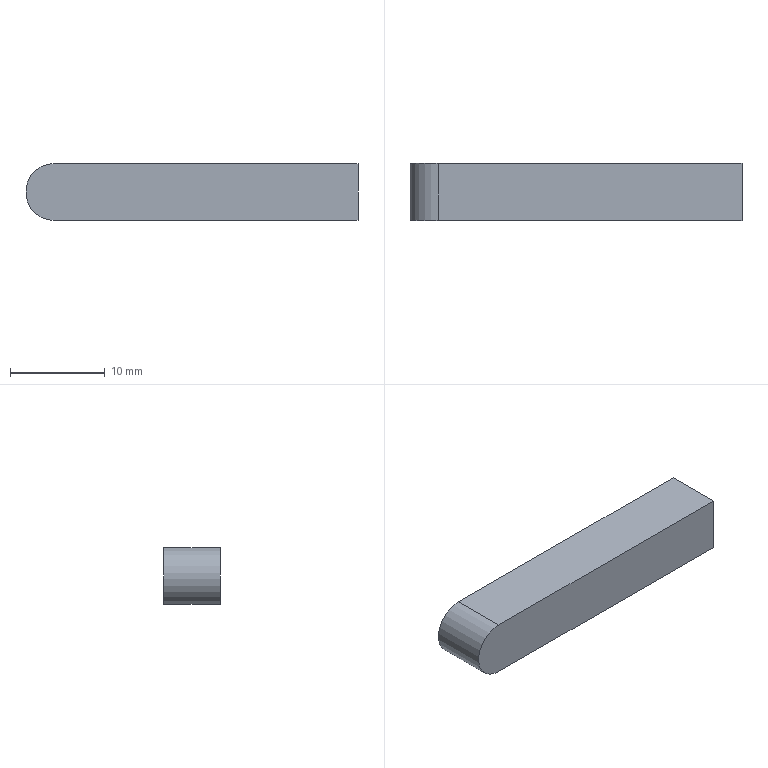Part | STEP file | G3L22N30-MM02TNNTNXH6-Part-5 | 1 solid | 6 faces | box 35 x 6 x 6 mm | volume 1237 mm3 | plane 5 | cylinder 1 | commonest cylinder face diameters 6 x1
STEP:
#1=CARTESIAN_POINT('',(40.,7.5,-3.));
#2=VERTEX_POINT('',#1);
#3=CARTESIAN_POINT('',(8.,7.5,-3.));
#4=VERTEX_POINT('',#3);
#5=CARTESIAN_POINT('',(40.,7.5,-3.));
#6=DIRECTION('',(-1.,0.,0.));
#7=VECTOR('',#6,1000.);
#8=LINE('',#5,#7);
#9=EDGE_CURVE('',#2,#4,#8,.T.);
#10=ORIENTED_EDGE('',*,*,#9,.T.);
#11=CARTESIAN_POINT('',(8.,13.5,-3.));
#12=VERTEX_POINT('',#11);
#13=CARTESIAN_POINT('',(8.,13.5,-3.));
#14=DIRECTION('',(0.,-1.,0.));
#15=VECTOR('',#14,1000.);
#16=LINE('',#13,#15);
#17=EDGE_CURVE('',#12,#4,#16,.T.);
#18=ORIENTED_EDGE('',*,*,#17,.F.);
#19=CARTESIAN_POINT('',(40.,13.5,-3.));
#20=VERTEX_POINT('',#19);
#21=CARTESIAN_POINT('',(40.,13.5,-3.));
#22=DIRECTION('',(-1.,0.,0.));
#23=VECTOR('',#22,1000.);
#24=LINE('',#21,#23);
#25=EDGE_CURVE('',#20,#12,#24,.T.);
#26=ORIENTED_EDGE('',*,*,#25,.F.);
#27=CARTESIAN_POINT('',(40.,13.5,-3.));
#28=DIRECTION('',(0.,-1.,0.));
#29=VECTOR('',#28,1000.);
#30=LINE('',#27,#29);
#31=EDGE_CURVE('',#20,#2,#30,.T.);
#32=ORIENTED_EDGE('',*,*,#31,.T.);
#33=EDGE_LOOP('',(#10,#18,#26,#32));
#34=FACE_OUTER_BOUND('',#33,.T.);
#35=CARTESIAN_POINT('',(40.,13.5,-3.));
#36=DIRECTION('',(0.,0.,1.));
#37=DIRECTION('',(1.,0.,0.));
#38=AXIS2_PLACEMENT_3D('',#35,#36,#37);
#39=PLANE('',#38);
#40=ADVANCED_FACE('',(#34),#39,.F.);
#41=CARTESIAN_POINT('',(8.,7.5,3.));
#42=VERTEX_POINT('',#41);
#43=CARTESIAN_POINT('',(8.,7.5,0.));
#44=DIRECTION('',(0.,1.,0.));
#45=DIRECTION('',(1.,0.,0.));
#46=AXIS2_PLACEMENT_3D('',#43,#44,#45);
#47=CIRCLE('',#46,3.);
#48=EDGE_CURVE('',#4,#42,#47,.T.);
#49=ORIENTED_EDGE('',*,*,#48,.T.);
#50=CARTESIAN_POINT('',(8.,13.5,3.));
#51=VERTEX_POINT('',#50);
#52=CARTESIAN_POINT('',(8.,13.5,3.));
#53=DIRECTION('',(0.,-1.,0.));
#54=VECTOR('',#53,1000.);
#55=LINE('',#52,#54);
#56=EDGE_CURVE('',#51,#42,#55,.T.);
#57=ORIENTED_EDGE('',*,*,#56,.F.);
#58=CARTESIAN_POINT('',(8.,13.5,0.));
#59=DIRECTION('',(0.,1.,0.));
#60=DIRECTION('',(1.,0.,0.));
#61=AXIS2_PLACEMENT_3D('',#58,#59,#60);
#62=CIRCLE('',#61,3.);
#63=EDGE_CURVE('',#12,#51,#62,.T.);
#64=ORIENTED_EDGE('',*,*,#63,.F.);
#65=ORIENTED_EDGE('',*,*,#17,.T.);
#66=EDGE_LOOP('',(#49,#57,#64,#65));
#67=FACE_OUTER_BOUND('',#66,.T.);
#68=CARTESIAN_POINT('',(8.,13.5,0.));
#69=DIRECTION('',(0.,-1.,0.));
#70=DIRECTION('',(0.,0.,-1.));
#71=AXIS2_PLACEMENT_3D('',#68,#69,#70);
#72=CYLINDRICAL_SURFACE('',#71,3.);
#73=ADVANCED_FACE('',(#67),#72,.T.);
#74=CARTESIAN_POINT('',(40.,7.5,3.));
#75=VERTEX_POINT('',#74);
#76=CARTESIAN_POINT('',(8.,7.5,3.));
#77=DIRECTION('',(1.,0.,0.));
#78=VECTOR('',#77,1000.);
#79=LINE('',#76,#78);
#80=EDGE_CURVE('',#42,#75,#79,.T.);
#81=ORIENTED_EDGE('',*,*,#80,.T.);
#82=CARTESIAN_POINT('',(40.,13.5,3.));
#83=VERTEX_POINT('',#82);
#84=CARTESIAN_POINT('',(40.,13.5,3.));
#85=DIRECTION('',(0.,-1.,0.));
#86=VECTOR('',#85,1000.);
#87=LINE('',#84,#86);
#88=EDGE_CURVE('',#83,#75,#87,.T.);
#89=ORIENTED_EDGE('',*,*,#88,.F.);
#90=CARTESIAN_POINT('',(8.,13.5,3.));
#91=DIRECTION('',(1.,0.,0.));
#92=VECTOR('',#91,1000.);
#93=LINE('',#90,#92);
#94=EDGE_CURVE('',#51,#83,#93,.T.);
#95=ORIENTED_EDGE('',*,*,#94,.F.);
#96=ORIENTED_EDGE('',*,*,#56,.T.);
#97=EDGE_LOOP('',(#81,#89,#95,#96));
#98=FACE_OUTER_BOUND('',#97,.T.);
#99=CARTESIAN_POINT('',(8.,13.5,3.));
#100=DIRECTION('',(0.,0.,-1.));
#101=DIRECTION('',(-1.,0.,0.));
#102=AXIS2_PLACEMENT_3D('',#99,#100,#101);
#103=PLANE('',#102);
#104=ADVANCED_FACE('',(#98),#103,.F.);
#105=CARTESIAN_POINT('',(40.,7.5,3.));
#106=DIRECTION('',(0.,0.,-1.));
#107=VECTOR('',#106,1000.);
#108=LINE('',#105,#107);
#109=EDGE_CURVE('',#75,#2,#108,.T.);
#110=ORIENTED_EDGE('',*,*,#109,.T.);
#111=ORIENTED_EDGE('',*,*,#31,.F.);
#112=CARTESIAN_POINT('',(40.,13.5,3.));
#113=DIRECTION('',(0.,0.,-1.));
#114=VECTOR('',#113,1000.);
#115=LINE('',#112,#114);
#116=EDGE_CURVE('',#83,#20,#115,.T.);
#117=ORIENTED_EDGE('',*,*,#116,.F.);
#118=ORIENTED_EDGE('',*,*,#88,.T.);
#119=EDGE_LOOP('',(#110,#111,#117,#118));
#120=FACE_OUTER_BOUND('',#119,.T.);
#121=CARTESIAN_POINT('',(40.,13.5,3.));
#122=DIRECTION('',(-1.,0.,0.));
#123=DIRECTION('',(0.,0.,1.));
#124=AXIS2_PLACEMENT_3D('',#121,#122,#123);
#125=PLANE('',#124);
#126=ADVANCED_FACE('',(#120),#125,.F.);
#127=ORIENTED_EDGE('',*,*,#25,.T.);
#128=ORIENTED_EDGE('',*,*,#63,.T.);
#129=ORIENTED_EDGE('',*,*,#94,.T.);
#130=ORIENTED_EDGE('',*,*,#116,.T.);
#131=EDGE_LOOP('',(#127,#128,#129,#130));
#132=FACE_OUTER_BOUND('',#131,.T.);
#133=CARTESIAN_POINT('',(8.,13.5,0.));
#134=DIRECTION('',(0.,1.,0.));
#135=DIRECTION('',(0.,0.,1.));
#136=AXIS2_PLACEMENT_3D('',#133,#134,#135);
#137=PLANE('',#136);
#138=ADVANCED_FACE('',(#132),#137,.T.);
#139=ORIENTED_EDGE('',*,*,#9,.F.);
#140=ORIENTED_EDGE('',*,*,#109,.F.);
#141=ORIENTED_EDGE('',*,*,#80,.F.);
#142=ORIENTED_EDGE('',*,*,#48,.F.);
#143=EDGE_LOOP('',(#139,#140,#141,#142));
#144=FACE_OUTER_BOUND('',#143,.T.);
#145=CARTESIAN_POINT('',(8.,7.5,0.));
#146=DIRECTION('',(0.,1.,0.));
#147=DIRECTION('',(0.,0.,1.));
#148=AXIS2_PLACEMENT_3D('',#145,#146,#147);
#149=PLANE('',#148);
#150=ADVANCED_FACE('',(#144),#149,.F.);
#151=CLOSED_SHELL('',(#40,#73,#104,#126,#138,#150));
#152=MANIFOLD_SOLID_BREP('',#151);
#153=CARTESIAN_POINT('',(0.,0.,0.));
#154=DIRECTION('',(0.,0.,1.));
#155=DIRECTION('',(1.,0.,0.));
#156=AXIS2_PLACEMENT_3D('',#153,#154,#155);
#157=(LENGTH_UNIT()NAMED_UNIT(*)SI_UNIT(.MILLI.,.METRE.));
#158=UNCERTAINTY_MEASURE_WITH_UNIT(LENGTH_MEASURE(0.00001),#157,'','');
#159=(NAMED_UNIT(*)PLANE_ANGLE_UNIT()SI_UNIT($,.RADIAN.));
#160=(NAMED_UNIT(*)SI_UNIT($,.STERADIAN.)SOLID_ANGLE_UNIT());
#161=(GEOMETRIC_REPRESENTATION_CONTEXT(3)GLOBAL_UNCERTAINTY_ASSIGNED_CONTEXT((#158))GLOBAL_UNIT_ASSIGNED_CONTEXT((#157,#159,#160))REPRESENTATION_CONTEXT('',''));
#162=ADVANCED_BREP_SHAPE_REPRESENTATION('',(#152,#156),#161);